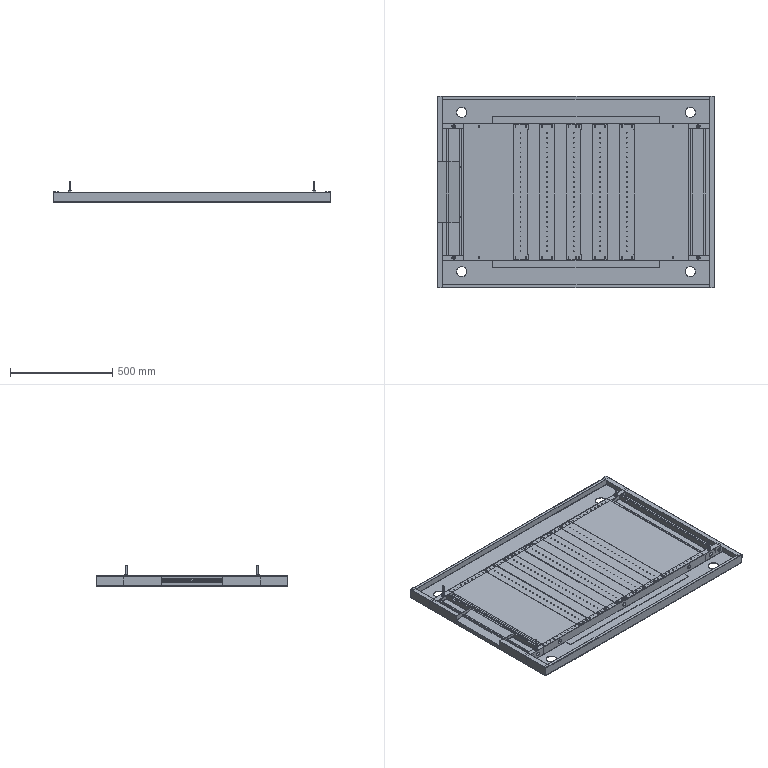Part | SolidWorks | features ReferencePattern 15, MirrorCompFeat 4, LocalLPattern 1 | 30 solids | 1411 faces | box 1360 x 940 x 103 mm | volume 5180100 mm3 | cylinder 753 | plane 598 | cone 56 | spline 4 | commonest cylinder face diameters 4.2 x501 20 x52 0.4 x42 6 x40 2.4 x36 8 x20